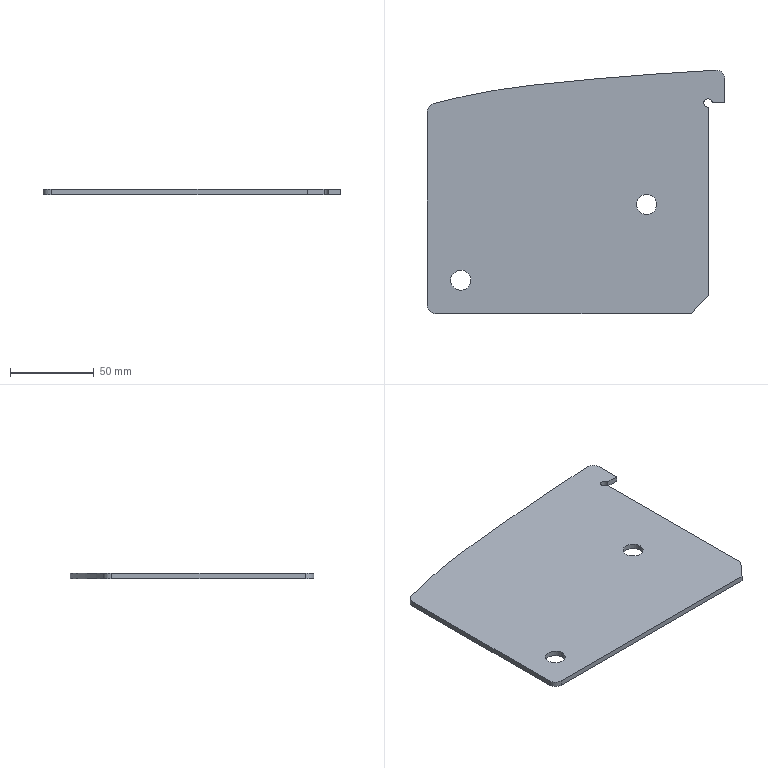Part | SolidWorks | features FlatPattern 1, SMBaseFlange 1, SheetMetal 1 | 1 solid | 19 faces | box 177.818 x 145.585 x 3.2 mm | volume 73602 mm3 | cylinder 11 | plane 8 | commonest cylinder face diameters 12 x4 10 x3 5 x2 796 x1 3976 x1
STEP:
#1=CARTESIAN_POINT('',(-150.,781.7,3.2));
#2=VERTEX_POINT('',#1);
#3=CARTESIAN_POINT('',(-138.,781.7,3.2));
#4=VERTEX_POINT('',#3);
#5=CARTESIAN_POINT('',(-144.,781.7,3.2));
#6=DIRECTION('',(0.,0.,1.));
#7=DIRECTION('',(1.,0.,0.));
#8=AXIS2_PLACEMENT_3D('',#5,#6,#7);
#9=CIRCLE('',#8,6.);
#10=EDGE_CURVE('',#2,#4,#9,.T.);
#11=ORIENTED_EDGE('',*,*,#10,.T.);
#12=CARTESIAN_POINT('',(-138.,781.7,0.));
#13=VERTEX_POINT('',#12);
#14=CARTESIAN_POINT('',(-138.,781.7,3.2));
#15=DIRECTION('',(0.,0.,-1.));
#16=VECTOR('',#15,1000.);
#17=LINE('',#14,#16);
#18=EDGE_CURVE('',#4,#13,#17,.T.);
#19=ORIENTED_EDGE('',*,*,#18,.T.);
#20=CARTESIAN_POINT('',(-150.,781.7,0.));
#21=VERTEX_POINT('',#20);
#22=CARTESIAN_POINT('',(-144.,781.7,0.));
#23=DIRECTION('',(0.,0.,1.));
#24=DIRECTION('',(1.,0.,0.));
#25=AXIS2_PLACEMENT_3D('',#22,#23,#24);
#26=CIRCLE('',#25,6.);
#27=EDGE_CURVE('',#21,#13,#26,.T.);
#28=ORIENTED_EDGE('',*,*,#27,.F.);
#29=CARTESIAN_POINT('',(-150.,781.7,3.2));
#30=DIRECTION('',(0.,0.,-1.));
#31=VECTOR('',#30,1000.);
#32=LINE('',#29,#31);
#33=EDGE_CURVE('',#2,#21,#32,.T.);
#34=ORIENTED_EDGE('',*,*,#33,.F.);
#35=EDGE_LOOP('',(#11,#19,#28,#34));
#36=FACE_OUTER_BOUND('',#35,.T.);
#37=CARTESIAN_POINT('',(-144.,781.7,3.2));
#38=DIRECTION('',(0.,0.,-1.));
#39=DIRECTION('',(-1.,0.,0.));
#40=AXIS2_PLACEMENT_3D('',#37,#38,#39);
#41=CYLINDRICAL_SURFACE('',#40,6.);
#42=ADVANCED_FACE('',(#36),#41,.F.);
#43=CARTESIAN_POINT('',(-38.896,827.041,3.2));
#44=VERTEX_POINT('',#43);
#45=CARTESIAN_POINT('',(-26.896,827.041,3.2));
#46=VERTEX_POINT('',#45);
#47=CARTESIAN_POINT('',(-32.896,827.041,3.2));
#48=DIRECTION('',(0.,0.,1.));
#49=DIRECTION('',(1.,0.,0.));
#50=AXIS2_PLACEMENT_3D('',#47,#48,#49);
#51=CIRCLE('',#50,6.);
#52=EDGE_CURVE('',#44,#46,#51,.T.);
#53=ORIENTED_EDGE('',*,*,#52,.T.);
#54=CARTESIAN_POINT('',(-26.896,827.041,0.));
#55=VERTEX_POINT('',#54);
#56=CARTESIAN_POINT('',(-26.896,827.041,3.2));
#57=DIRECTION('',(0.,0.,-1.));
#58=VECTOR('',#57,1000.);
#59=LINE('',#56,#58);
#60=EDGE_CURVE('',#46,#55,#59,.T.);
#61=ORIENTED_EDGE('',*,*,#60,.T.);
#62=CARTESIAN_POINT('',(-38.896,827.041,0.));
#63=VERTEX_POINT('',#62);
#64=CARTESIAN_POINT('',(-32.896,827.041,0.));
#65=DIRECTION('',(0.,0.,1.));
#66=DIRECTION('',(1.,0.,0.));
#67=AXIS2_PLACEMENT_3D('',#64,#65,#66);
#68=CIRCLE('',#67,6.);
#69=EDGE_CURVE('',#63,#55,#68,.T.);
#70=ORIENTED_EDGE('',*,*,#69,.F.);
#71=CARTESIAN_POINT('',(-38.896,827.041,3.2));
#72=DIRECTION('',(0.,0.,-1.));
#73=VECTOR('',#72,1000.);
#74=LINE('',#71,#73);
#75=EDGE_CURVE('',#44,#63,#74,.T.);
#76=ORIENTED_EDGE('',*,*,#75,.F.);
#77=EDGE_LOOP('',(#53,#61,#70,#76));
#78=FACE_OUTER_BOUND('',#77,.T.);
#79=CARTESIAN_POINT('',(-32.896,827.041,3.2));
#80=DIRECTION('',(0.,0.,-1.));
#81=DIRECTION('',(-1.,0.,0.));
#82=AXIS2_PLACEMENT_3D('',#79,#80,#81);
#83=CYLINDRICAL_SURFACE('',#82,6.);
#84=ADVANCED_FACE('',(#78),#83,.F.);
#85=CARTESIAN_POINT('',(1.318,887.697,3.2));
#86=VERTEX_POINT('',#85);
#87=CARTESIAN_POINT('',(6.318,887.697,3.2));
#88=VERTEX_POINT('',#87);
#89=CARTESIAN_POINT('',(3.818,887.697,3.2));
#90=DIRECTION('',(0.,0.,-1.));
#91=DIRECTION('',(1.,0.,0.));
#92=AXIS2_PLACEMENT_3D('',#89,#90,#91);
#93=CIRCLE('',#92,2.5);
#94=EDGE_CURVE('',#86,#88,#93,.T.);
#95=ORIENTED_EDGE('',*,*,#94,.F.);
#96=CARTESIAN_POINT('',(1.318,887.697,0.));
#97=VERTEX_POINT('',#96);
#98=CARTESIAN_POINT('',(1.318,887.697,3.2));
#99=DIRECTION('',(0.,0.,-1.));
#100=VECTOR('',#99,1000.);
#101=LINE('',#98,#100);
#102=EDGE_CURVE('',#86,#97,#101,.T.);
#103=ORIENTED_EDGE('',*,*,#102,.T.);
#104=CARTESIAN_POINT('',(6.318,887.697,0.));
#105=VERTEX_POINT('',#104);
#106=CARTESIAN_POINT('',(3.818,887.697,0.));
#107=DIRECTION('',(0.,0.,-1.));
#108=DIRECTION('',(1.,0.,0.));
#109=AXIS2_PLACEMENT_3D('',#106,#107,#108);
#110=CIRCLE('',#109,2.5);
#111=EDGE_CURVE('',#97,#105,#110,.T.);
#112=ORIENTED_EDGE('',*,*,#111,.T.);
#113=CARTESIAN_POINT('',(6.318,887.697,3.2));
#114=DIRECTION('',(0.,0.,-1.));
#115=VECTOR('',#114,1000.);
#116=LINE('',#113,#115);
#117=EDGE_CURVE('',#88,#105,#116,.T.);
#118=ORIENTED_EDGE('',*,*,#117,.F.);
#119=EDGE_LOOP('',(#95,#103,#112,#118));
#120=FACE_OUTER_BOUND('',#119,.T.);
#121=CARTESIAN_POINT('',(3.818,887.697,3.2));
#122=DIRECTION('',(0.,0.,-1.));
#123=DIRECTION('',(-1.,0.,0.));
#124=AXIS2_PLACEMENT_3D('',#121,#122,#123);
#125=CYLINDRICAL_SURFACE('',#124,2.5);
#126=ADVANCED_FACE('',(#120),#125,.F.);
#127=ORIENTED_EDGE('',*,*,#52,.F.);
#128=CARTESIAN_POINT('',(-32.896,827.041,3.2));
#129=DIRECTION('',(0.,0.,1.));
#130=DIRECTION('',(1.,0.,0.));
#131=AXIS2_PLACEMENT_3D('',#128,#129,#130);
#132=CIRCLE('',#131,6.);
#133=EDGE_CURVE('',#46,#44,#132,.T.);
#134=ORIENTED_EDGE('',*,*,#133,.F.);
#135=EDGE_LOOP('',(#127,#134));
#136=FACE_BOUND('',#135,.T.);
#137=CARTESIAN_POINT('',(13.818,887.697,3.2));
#138=VERTEX_POINT('',#137);
#139=CARTESIAN_POINT('',(13.818,902.285,3.2));
#140=VERTEX_POINT('',#139);
#141=CARTESIAN_POINT('',(13.818,887.697,3.2));
#142=DIRECTION('',(0.,1.,0.));
#143=VECTOR('',#142,1000.);
#144=LINE('',#141,#143);
#145=EDGE_CURVE('',#138,#140,#144,.T.);
#146=ORIENTED_EDGE('',*,*,#145,.T.);
#147=CARTESIAN_POINT('',(8.551,907.278,3.2));
#148=VERTEX_POINT('',#147);
#149=CARTESIAN_POINT('',(8.818,902.285,3.2));
#150=DIRECTION('',(0.,0.,1.));
#151=DIRECTION('',(1.,0.,0.));
#152=AXIS2_PLACEMENT_3D('',#149,#150,#151);
#153=CIRCLE('',#152,5.);
#154=EDGE_CURVE('',#140,#148,#153,.T.);
#155=ORIENTED_EDGE('',*,*,#154,.T.);
#156=CARTESIAN_POINT('',(-101.22,898.356,3.2));
#157=VERTEX_POINT('',#156);
#158=CARTESIAN_POINT('',(114.664,-1077.888,3.2));
#159=DIRECTION('',(0.,0.,1.));
#160=DIRECTION('',(1.,0.,0.));
#161=AXIS2_PLACEMENT_3D('',#158,#159,#160);
#162=CIRCLE('',#161,1988.);
#163=EDGE_CURVE('',#148,#157,#162,.T.);
#164=ORIENTED_EDGE('',*,*,#163,.T.);
#165=CARTESIAN_POINT('',(-160.285,887.341,3.2));
#166=VERTEX_POINT('',#165);
#167=CARTESIAN_POINT('',(-58.,502.709,3.2));
#168=DIRECTION('',(0.,0.,1.));
#169=DIRECTION('',(1.,0.,0.));
#170=AXIS2_PLACEMENT_3D('',#167,#168,#169);
#171=CIRCLE('',#170,398.);
#172=EDGE_CURVE('',#157,#166,#171,.T.);
#173=ORIENTED_EDGE('',*,*,#172,.T.);
#174=CARTESIAN_POINT('',(-164.,882.509,3.2));
#175=VERTEX_POINT('',#174);
#176=CARTESIAN_POINT('',(-159.,882.509,3.2));
#177=DIRECTION('',(0.,0.,1.));
#178=DIRECTION('',(-1.,0.,0.));
#179=AXIS2_PLACEMENT_3D('',#176,#177,#178);
#180=CIRCLE('',#179,5.);
#181=EDGE_CURVE('',#166,#175,#180,.T.);
#182=ORIENTED_EDGE('',*,*,#181,.T.);
#183=CARTESIAN_POINT('',(-164.,766.7,3.2));
#184=VERTEX_POINT('',#183);
#185=CARTESIAN_POINT('',(-164.,766.7,3.2));
#186=DIRECTION('',(0.,-1.,0.));
#187=VECTOR('',#186,1000.);
#188=LINE('',#185,#187);
#189=EDGE_CURVE('',#175,#184,#188,.T.);
#190=ORIENTED_EDGE('',*,*,#189,.T.);
#191=CARTESIAN_POINT('',(-159.,761.7,3.2));
#192=VERTEX_POINT('',#191);
#193=CARTESIAN_POINT('',(-159.,766.7,3.2));
#194=DIRECTION('',(0.,0.,1.));
#195=DIRECTION('',(-1.,0.,0.));
#196=AXIS2_PLACEMENT_3D('',#193,#194,#195);
#197=CIRCLE('',#196,5.);
#198=EDGE_CURVE('',#184,#192,#197,.T.);
#199=ORIENTED_EDGE('',*,*,#198,.T.);
#200=CARTESIAN_POINT('',(-6.182,761.7,3.2));
#201=VERTEX_POINT('',#200);
#202=CARTESIAN_POINT('',(-6.182,761.7,3.2));
#203=DIRECTION('',(1.,0.,0.));
#204=VECTOR('',#203,1000.);
#205=LINE('',#202,#204);
#206=EDGE_CURVE('',#192,#201,#205,.T.);
#207=ORIENTED_EDGE('',*,*,#206,.T.);
#208=CARTESIAN_POINT('',(3.818,772.697,3.2));
#209=VERTEX_POINT('',#208);
#210=CARTESIAN_POINT('',(3.818,772.697,3.2));
#211=DIRECTION('',(0.6728,0.7398,0.));
#212=VECTOR('',#211,1000.);
#213=LINE('',#210,#212);
#214=EDGE_CURVE('',#201,#209,#213,.T.);
#215=ORIENTED_EDGE('',*,*,#214,.T.);
#216=CARTESIAN_POINT('',(3.818,885.197,3.2));
#217=VERTEX_POINT('',#216);
#218=CARTESIAN_POINT('',(3.818,885.197,3.2));
#219=DIRECTION('',(0.,1.,0.));
#220=VECTOR('',#219,1000.);
#221=LINE('',#218,#220);
#222=EDGE_CURVE('',#209,#217,#221,.T.);
#223=ORIENTED_EDGE('',*,*,#222,.T.);
#224=CARTESIAN_POINT('',(3.818,887.697,3.2));
#225=DIRECTION('',(0.,0.,-1.));
#226=DIRECTION('',(1.,0.,0.));
#227=AXIS2_PLACEMENT_3D('',#224,#225,#226);
#228=CIRCLE('',#227,2.5);
#229=EDGE_CURVE('',#217,#86,#228,.T.);
#230=ORIENTED_EDGE('',*,*,#229,.T.);
#231=ORIENTED_EDGE('',*,*,#94,.T.);
#232=CARTESIAN_POINT('',(6.318,887.697,3.2));
#233=DIRECTION('',(1.,0.,0.));
#234=VECTOR('',#233,1000.);
#235=LINE('',#232,#234);
#236=EDGE_CURVE('',#88,#138,#235,.T.);
#237=ORIENTED_EDGE('',*,*,#236,.T.);
#238=EDGE_LOOP('',(#146,#155,#164,#173,#182,#190,#199,#207,#215,#223,#230,#231,#237));
#239=FACE_OUTER_BOUND('',#238,.T.);
#240=ORIENTED_EDGE('',*,*,#10,.F.);
#241=CARTESIAN_POINT('',(-144.,781.7,3.2));
#242=DIRECTION('',(0.,0.,1.));
#243=DIRECTION('',(1.,0.,0.));
#244=AXIS2_PLACEMENT_3D('',#241,#242,#243);
#245=CIRCLE('',#244,6.);
#246=EDGE_CURVE('',#4,#2,#245,.T.);
#247=ORIENTED_EDGE('',*,*,#246,.F.);
#248=EDGE_LOOP('',(#240,#247));
#249=FACE_BOUND('',#248,.T.);
#250=CARTESIAN_POINT('',(8.818,902.285,3.2));
#251=DIRECTION('',(0.,0.,1.));
#252=DIRECTION('',(1.,0.,0.));
#253=AXIS2_PLACEMENT_3D('',#250,#251,#252);
#254=PLANE('',#253);
#255=ADVANCED_FACE('',(#136,#239,#249),#254,.T.);
#256=CARTESIAN_POINT('',(13.818,887.697,0.));
#257=VERTEX_POINT('',#256);
#258=CARTESIAN_POINT('',(13.818,902.285,0.));
#259=VERTEX_POINT('',#258);
#260=CARTESIAN_POINT('',(13.818,887.697,0.));
#261=DIRECTION('',(0.,1.,0.));
#262=VECTOR('',#261,1000.);
#263=LINE('',#260,#262);
#264=EDGE_CURVE('',#257,#259,#263,.T.);
#265=ORIENTED_EDGE('',*,*,#264,.F.);
#266=CARTESIAN_POINT('',(6.318,887.697,0.));
#267=DIRECTION('',(1.,0.,0.));
#268=VECTOR('',#267,1000.);
#269=LINE('',#266,#268);
#270=EDGE_CURVE('',#105,#257,#269,.T.);
#271=ORIENTED_EDGE('',*,*,#270,.F.);
#272=ORIENTED_EDGE('',*,*,#111,.F.);
#273=CARTESIAN_POINT('',(3.818,885.197,0.));
#274=VERTEX_POINT('',#273);
#275=CARTESIAN_POINT('',(3.818,887.697,0.));
#276=DIRECTION('',(0.,0.,-1.));
#277=DIRECTION('',(1.,0.,0.));
#278=AXIS2_PLACEMENT_3D('',#275,#276,#277);
#279=CIRCLE('',#278,2.5);
#280=EDGE_CURVE('',#274,#97,#279,.T.);
#281=ORIENTED_EDGE('',*,*,#280,.F.);
#282=CARTESIAN_POINT('',(3.818,772.697,0.));
#283=VERTEX_POINT('',#282);
#284=CARTESIAN_POINT('',(3.818,885.197,0.));
#285=DIRECTION('',(0.,1.,0.));
#286=VECTOR('',#285,1000.);
#287=LINE('',#284,#286);
#288=EDGE_CURVE('',#283,#274,#287,.T.);
#289=ORIENTED_EDGE('',*,*,#288,.F.);
#290=CARTESIAN_POINT('',(-6.182,761.7,0.));
#291=VERTEX_POINT('',#290);
#292=CARTESIAN_POINT('',(3.818,772.697,0.));
#293=DIRECTION('',(0.6728,0.7398,0.));
#294=VECTOR('',#293,1000.);
#295=LINE('',#292,#294);
#296=EDGE_CURVE('',#291,#283,#295,.T.);
#297=ORIENTED_EDGE('',*,*,#296,.F.);
#298=CARTESIAN_POINT('',(-159.,761.7,0.));
#299=VERTEX_POINT('',#298);
#300=CARTESIAN_POINT('',(-6.182,761.7,0.));
#301=DIRECTION('',(1.,0.,0.));
#302=VECTOR('',#301,1000.);
#303=LINE('',#300,#302);
#304=EDGE_CURVE('',#299,#291,#303,.T.);
#305=ORIENTED_EDGE('',*,*,#304,.F.);
#306=CARTESIAN_POINT('',(-164.,766.7,0.));
#307=VERTEX_POINT('',#306);
#308=CARTESIAN_POINT('',(-159.,766.7,0.));
#309=DIRECTION('',(0.,0.,1.));
#310=DIRECTION('',(-1.,0.,0.));
#311=AXIS2_PLACEMENT_3D('',#308,#309,#310);
#312=CIRCLE('',#311,5.);
#313=EDGE_CURVE('',#307,#299,#312,.T.);
#314=ORIENTED_EDGE('',*,*,#313,.F.);
#315=CARTESIAN_POINT('',(-164.,882.509,0.));
#316=VERTEX_POINT('',#315);
#317=CARTESIAN_POINT('',(-164.,766.7,0.));
#318=DIRECTION('',(0.,-1.,0.));
#319=VECTOR('',#318,1000.);
#320=LINE('',#317,#319);
#321=EDGE_CURVE('',#316,#307,#320,.T.);
#322=ORIENTED_EDGE('',*,*,#321,.F.);
#323=CARTESIAN_POINT('',(-160.285,887.341,0.));
#324=VERTEX_POINT('',#323);
#325=CARTESIAN_POINT('',(-159.,882.509,0.));
#326=DIRECTION('',(0.,0.,1.));
#327=DIRECTION('',(-1.,0.,0.));
#328=AXIS2_PLACEMENT_3D('',#325,#326,#327);
#329=CIRCLE('',#328,5.);
#330=EDGE_CURVE('',#324,#316,#329,.T.);
#331=ORIENTED_EDGE('',*,*,#330,.F.);
#332=CARTESIAN_POINT('',(-101.22,898.356,0.));
#333=VERTEX_POINT('',#332);
#334=CARTESIAN_POINT('',(-58.,502.709,0.));
#335=DIRECTION('',(0.,0.,1.));
#336=DIRECTION('',(1.,0.,0.));
#337=AXIS2_PLACEMENT_3D('',#334,#335,#336);
#338=CIRCLE('',#337,398.);
#339=EDGE_CURVE('',#333,#324,#338,.T.);
#340=ORIENTED_EDGE('',*,*,#339,.F.);
#341=CARTESIAN_POINT('',(8.551,907.278,0.));
#342=VERTEX_POINT('',#341);
#343=CARTESIAN_POINT('',(114.664,-1077.888,0.));
#344=DIRECTION('',(0.,0.,1.));
#345=DIRECTION('',(1.,0.,0.));
#346=AXIS2_PLACEMENT_3D('',#343,#344,#345);
#347=CIRCLE('',#346,1988.);
#348=EDGE_CURVE('',#342,#333,#347,.T.);
#349=ORIENTED_EDGE('',*,*,#348,.F.);
#350=CARTESIAN_POINT('',(8.818,902.285,0.));
#351=DIRECTION('',(0.,0.,1.));
#352=DIRECTION('',(1.,0.,0.));
#353=AXIS2_PLACEMENT_3D('',#350,#351,#352);
#354=CIRCLE('',#353,5.);
#355=EDGE_CURVE('',#259,#342,#354,.T.);
#356=ORIENTED_EDGE('',*,*,#355,.F.);
#357=EDGE_LOOP('',(#265,#271,#272,#281,#289,#297,#305,#314,#322,#331,#340,#349,#356));
#358=FACE_OUTER_BOUND('',#357,.T.);
#359=ORIENTED_EDGE('',*,*,#69,.T.);
#360=CARTESIAN_POINT('',(-32.896,827.041,0.));
#361=DIRECTION('',(0.,0.,1.));
#362=DIRECTION('',(1.,0.,0.));
#363=AXIS2_PLACEMENT_3D('',#360,#361,#362);
#364=CIRCLE('',#363,6.);
#365=EDGE_CURVE('',#55,#63,#364,.T.);
#366=ORIENTED_EDGE('',*,*,#365,.T.);
#367=EDGE_LOOP('',(#359,#366));
#368=FACE_BOUND('',#367,.T.);
#369=ORIENTED_EDGE('',*,*,#27,.T.);
#370=CARTESIAN_POINT('',(-144.,781.7,0.));
#371=DIRECTION('',(0.,0.,1.));
#372=DIRECTION('',(1.,0.,0.));
#373=AXIS2_PLACEMENT_3D('',#370,#371,#372);
#374=CIRCLE('',#373,6.);
#375=EDGE_CURVE('',#13,#21,#374,.T.);
#376=ORIENTED_EDGE('',*,*,#375,.T.);
#377=EDGE_LOOP('',(#369,#376));
#378=FACE_BOUND('',#377,.T.);
#379=CARTESIAN_POINT('',(8.818,902.285,0.));
#380=DIRECTION('',(0.,0.,1.));
#381=DIRECTION('',(1.,0.,0.));
#382=AXIS2_PLACEMENT_3D('',#379,#380,#381);
#383=PLANE('',#382);
#384=ADVANCED_FACE('',(#358,#368,#378),#383,.F.);
#385=ORIENTED_EDGE('',*,*,#264,.T.);
#386=CARTESIAN_POINT('',(13.818,902.285,3.2));
#387=DIRECTION('',(0.,0.,-1.));
#388=VECTOR('',#387,1000.);
#389=LINE('',#386,#388);
#390=EDGE_CURVE('',#140,#259,#389,.T.);
#391=ORIENTED_EDGE('',*,*,#390,.F.);
#392=ORIENTED_EDGE('',*,*,#145,.F.);
#393=CARTESIAN_POINT('',(13.818,887.697,3.2));
#394=DIRECTION('',(0.,0.,-1.));
#395=VECTOR('',#394,1000.);
#396=LINE('',#393,#395);
#397=EDGE_CURVE('',#138,#257,#396,.T.);
#398=ORIENTED_EDGE('',*,*,#397,.T.);
#399=EDGE_LOOP('',(#385,#391,#392,#398));
#400=FACE_OUTER_BOUND('',#399,.T.);
#401=CARTESIAN_POINT('',(13.818,887.697,3.2));
#402=DIRECTION('',(-1.,0.,0.));
#403=DIRECTION('',(0.,0.,1.));
#404=AXIS2_PLACEMENT_3D('',#401,#402,#403);
#405=PLANE('',#404);
#406=ADVANCED_FACE('',(#400),#405,.F.);
#407=ORIENTED_EDGE('',*,*,#355,.T.);
#408=CARTESIAN_POINT('',(8.551,907.278,3.2));
#409=DIRECTION('',(0.,0.,-1.));
#410=VECTOR('',#409,1000.);
#411=LINE('',#408,#410);
#412=EDGE_CURVE('',#148,#342,#411,.T.);
#413=ORIENTED_EDGE('',*,*,#412,.F.);
#414=ORIENTED_EDGE('',*,*,#154,.F.);
#415=ORIENTED_EDGE('',*,*,#390,.T.);
#416=EDGE_LOOP('',(#407,#413,#414,#415));
#417=FACE_OUTER_BOUND('',#416,.T.);
#418=CARTESIAN_POINT('',(8.818,902.285,3.2));
#419=DIRECTION('',(0.,0.,-1.));
#420=DIRECTION('',(-1.,0.,0.));
#421=AXIS2_PLACEMENT_3D('',#418,#419,#420);
#422=CYLINDRICAL_SURFACE('',#421,5.);
#423=ADVANCED_FACE('',(#417),#422,.T.);
#424=ORIENTED_EDGE('',*,*,#348,.T.);
#425=CARTESIAN_POINT('',(-101.22,898.356,3.2));
#426=DIRECTION('',(0.,0.,-1.));
#427=VECTOR('',#426,1000.);
#428=LINE('',#425,#427);
#429=EDGE_CURVE('',#157,#333,#428,.T.);
#430=ORIENTED_EDGE('',*,*,#429,.F.);
#431=ORIENTED_EDGE('',*,*,#163,.F.);
#432=ORIENTED_EDGE('',*,*,#412,.T.);
#433=EDGE_LOOP('',(#424,#430,#431,#432));
#434=FACE_OUTER_BOUND('',#433,.T.);
#435=CARTESIAN_POINT('',(114.664,-1077.888,3.2));
#436=DIRECTION('',(0.,0.,-1.));
#437=DIRECTION('',(-1.,0.,0.));
#438=AXIS2_PLACEMENT_3D('',#435,#436,#437);
#439=CYLINDRICAL_SURFACE('',#438,1988.);
#440=ADVANCED_FACE('',(#434),#439,.T.);
#441=ORIENTED_EDGE('',*,*,#339,.T.);
#442=CARTESIAN_POINT('',(-160.285,887.341,3.2));
#443=DIRECTION('',(0.,0.,-1.));
#444=VECTOR('',#443,1000.);
#445=LINE('',#442,#444);
#446=EDGE_CURVE('',#166,#324,#445,.T.);
#447=ORIENTED_EDGE('',*,*,#446,.F.);
#448=ORIENTED_EDGE('',*,*,#172,.F.);
#449=ORIENTED_EDGE('',*,*,#429,.T.);
#450=EDGE_LOOP('',(#441,#447,#448,#449));
#451=FACE_OUTER_BOUND('',#450,.T.);
#452=CARTESIAN_POINT('',(-58.,502.709,3.2));
#453=DIRECTION('',(0.,0.,-1.));
#454=DIRECTION('',(-1.,0.,0.));
#455=AXIS2_PLACEMENT_3D('',#452,#453,#454);
#456=CYLINDRICAL_SURFACE('',#455,398.);
#457=ADVANCED_FACE('',(#451),#456,.T.);
#458=ORIENTED_EDGE('',*,*,#330,.T.);
#459=CARTESIAN_POINT('',(-164.,882.509,3.2));
#460=DIRECTION('',(0.,0.,-1.));
#461=VECTOR('',#460,1000.);
#462=LINE('',#459,#461);
#463=EDGE_CURVE('',#175,#316,#462,.T.);
#464=ORIENTED_EDGE('',*,*,#463,.F.);
#465=ORIENTED_EDGE('',*,*,#181,.F.);
#466=ORIENTED_EDGE('',*,*,#446,.T.);
#467=EDGE_LOOP('',(#458,#464,#465,#466));
#468=FACE_OUTER_BOUND('',#467,.T.);
#469=CARTESIAN_POINT('',(-159.,882.509,3.2));
#470=DIRECTION('',(0.,0.,-1.));
#471=DIRECTION('',(-1.,0.,0.));
#472=AXIS2_PLACEMENT_3D('',#469,#470,#471);
#473=CYLINDRICAL_SURFACE('',#472,5.);
#474=ADVANCED_FACE('',(#468),#473,.T.);
#475=ORIENTED_EDGE('',*,*,#321,.T.);
#476=CARTESIAN_POINT('',(-164.,766.7,3.2));
#477=DIRECTION('',(0.,0.,-1.));
#478=VECTOR('',#477,1000.);
#479=LINE('',#476,#478);
#480=EDGE_CURVE('',#184,#307,#479,.T.);
#481=ORIENTED_EDGE('',*,*,#480,.F.);
#482=ORIENTED_EDGE('',*,*,#189,.F.);
#483=ORIENTED_EDGE('',*,*,#463,.T.);
#484=EDGE_LOOP('',(#475,#481,#482,#483));
#485=FACE_OUTER_BOUND('',#484,.T.);
#486=CARTESIAN_POINT('',(-164.,766.7,3.2));
#487=DIRECTION('',(1.,0.,0.));
#488=DIRECTION('',(0.,0.,-1.));
#489=AXIS2_PLACEMENT_3D('',#486,#487,#488);
#490=PLANE('',#489);
#491=ADVANCED_FACE('',(#485),#490,.F.);
#492=ORIENTED_EDGE('',*,*,#313,.T.);
#493=CARTESIAN_POINT('',(-159.,761.7,3.2));
#494=DIRECTION('',(0.,0.,-1.));
#495=VECTOR('',#494,1000.);
#496=LINE('',#493,#495);
#497=EDGE_CURVE('',#192,#299,#496,.T.);
#498=ORIENTED_EDGE('',*,*,#497,.F.);
#499=ORIENTED_EDGE('',*,*,#198,.F.);
#500=ORIENTED_EDGE('',*,*,#480,.T.);
#501=EDGE_LOOP('',(#492,#498,#499,#500));
#502=FACE_OUTER_BOUND('',#501,.T.);
#503=CARTESIAN_POINT('',(-159.,766.7,3.2));
#504=DIRECTION('',(0.,0.,-1.));
#505=DIRECTION('',(-1.,0.,0.));
#506=AXIS2_PLACEMENT_3D('',#503,#504,#505);
#507=CYLINDRICAL_SURFACE('',#506,5.);
#508=ADVANCED_FACE('',(#502),#507,.T.);
#509=ORIENTED_EDGE('',*,*,#304,.T.);
#510=CARTESIAN_POINT('',(-6.182,761.7,3.2));
#511=DIRECTION('',(0.,0.,-1.));
#512=VECTOR('',#511,1000.);
#513=LINE('',#510,#512);
#514=EDGE_CURVE('',#201,#291,#513,.T.);
#515=ORIENTED_EDGE('',*,*,#514,.F.);
#516=ORIENTED_EDGE('',*,*,#206,.F.);
#517=ORIENTED_EDGE('',*,*,#497,.T.);
#518=EDGE_LOOP('',(#509,#515,#516,#517));
#519=FACE_OUTER_BOUND('',#518,.T.);
#520=CARTESIAN_POINT('',(-6.182,761.7,3.2));
#521=DIRECTION('',(0.,1.,0.));
#522=DIRECTION('',(0.,0.,1.));
#523=AXIS2_PLACEMENT_3D('',#520,#521,#522);
#524=PLANE('',#523);
#525=ADVANCED_FACE('',(#519),#524,.F.);
#526=ORIENTED_EDGE('',*,*,#296,.T.);
#527=CARTESIAN_POINT('',(3.818,772.697,3.2));
#528=DIRECTION('',(0.,0.,-1.));
#529=VECTOR('',#528,1000.);
#530=LINE('',#527,#529);
#531=EDGE_CURVE('',#209,#283,#530,.T.);
#532=ORIENTED_EDGE('',*,*,#531,.F.);
#533=ORIENTED_EDGE('',*,*,#214,.F.);
#534=ORIENTED_EDGE('',*,*,#514,.T.);
#535=EDGE_LOOP('',(#526,#532,#533,#534));
#536=FACE_OUTER_BOUND('',#535,.T.);
#537=CARTESIAN_POINT('',(3.818,772.697,3.2));
#538=DIRECTION('',(-0.7398,0.6728,0.));
#539=DIRECTION('',(-0.6728,-0.7398,0.));
#540=AXIS2_PLACEMENT_3D('',#537,#538,#539);
#541=PLANE('',#540);
#542=ADVANCED_FACE('',(#536),#541,.F.);
#543=ORIENTED_EDGE('',*,*,#288,.T.);
#544=CARTESIAN_POINT('',(3.818,885.197,3.2));
#545=DIRECTION('',(0.,0.,-1.));
#546=VECTOR('',#545,1000.);
#547=LINE('',#544,#546);
#548=EDGE_CURVE('',#217,#274,#547,.T.);
#549=ORIENTED_EDGE('',*,*,#548,.F.);
#550=ORIENTED_EDGE('',*,*,#222,.F.);
#551=ORIENTED_EDGE('',*,*,#531,.T.);
#552=EDGE_LOOP('',(#543,#549,#550,#551));
#553=FACE_OUTER_BOUND('',#552,.T.);
#554=CARTESIAN_POINT('',(3.818,885.197,3.2));
#555=DIRECTION('',(-1.,0.,0.));
#556=DIRECTION('',(0.,-1.,0.));
#557=AXIS2_PLACEMENT_3D('',#554,#555,#556);
#558=PLANE('',#557);
#559=ADVANCED_FACE('',(#553),#558,.F.);
#560=ORIENTED_EDGE('',*,*,#102,.F.);
#561=ORIENTED_EDGE('',*,*,#229,.F.);
#562=ORIENTED_EDGE('',*,*,#548,.T.);
#563=ORIENTED_EDGE('',*,*,#280,.T.);
#564=EDGE_LOOP('',(#560,#561,#562,#563));
#565=FACE_OUTER_BOUND('',#564,.T.);
#566=CARTESIAN_POINT('',(3.818,887.697,3.2));
#567=DIRECTION('',(0.,0.,-1.));
#568=DIRECTION('',(-1.,0.,0.));
#569=AXIS2_PLACEMENT_3D('',#566,#567,#568);
#570=CYLINDRICAL_SURFACE('',#569,2.5);
#571=ADVANCED_FACE('',(#565),#570,.F.);
#572=ORIENTED_EDGE('',*,*,#270,.T.);
#573=ORIENTED_EDGE('',*,*,#397,.F.);
#574=ORIENTED_EDGE('',*,*,#236,.F.);
#575=ORIENTED_EDGE('',*,*,#117,.T.);
#576=EDGE_LOOP('',(#572,#573,#574,#575));
#577=FACE_OUTER_BOUND('',#576,.T.);
#578=CARTESIAN_POINT('',(6.318,887.697,3.2));
#579=DIRECTION('',(0.,1.,0.));
#580=DIRECTION('',(0.,0.,1.));
#581=AXIS2_PLACEMENT_3D('',#578,#579,#580);
#582=PLANE('',#581);
#583=ADVANCED_FACE('',(#577),#582,.F.);
#584=ORIENTED_EDGE('',*,*,#60,.F.);
#585=ORIENTED_EDGE('',*,*,#133,.T.);
#586=ORIENTED_EDGE('',*,*,#75,.T.);
#587=ORIENTED_EDGE('',*,*,#365,.F.);
#588=EDGE_LOOP('',(#584,#585,#586,#587));
#589=FACE_OUTER_BOUND('',#588,.T.);
#590=CARTESIAN_POINT('',(-32.896,827.041,3.2));
#591=DIRECTION('',(0.,0.,-1.));
#592=DIRECTION('',(-1.,0.,0.));
#593=AXIS2_PLACEMENT_3D('',#590,#591,#592);
#594=CYLINDRICAL_SURFACE('',#593,6.);
#595=ADVANCED_FACE('',(#589),#594,.F.);
#596=ORIENTED_EDGE('',*,*,#18,.F.);
#597=ORIENTED_EDGE('',*,*,#246,.T.);
#598=ORIENTED_EDGE('',*,*,#33,.T.);
#599=ORIENTED_EDGE('',*,*,#375,.F.);
#600=EDGE_LOOP('',(#596,#597,#598,#599));
#601=FACE_OUTER_BOUND('',#600,.T.);
#602=CARTESIAN_POINT('',(-144.,781.7,3.2));
#603=DIRECTION('',(0.,0.,-1.));
#604=DIRECTION('',(-1.,0.,0.));
#605=AXIS2_PLACEMENT_3D('',#602,#603,#604);
#606=CYLINDRICAL_SURFACE('',#605,6.);
#607=ADVANCED_FACE('',(#601),#606,.F.);
#608=CLOSED_SHELL('',(#42,#84,#126,#255,#384,#406,#423,#440,#457,#474,#491,#508,#525,#542,#559,#571,#583,#595,#607));
#609=MANIFOLD_SOLID_BREP('',#608);
#610=CARTESIAN_POINT('',(0.,0.,0.));
#611=DIRECTION('',(0.,0.,1.));
#612=DIRECTION('',(1.,0.,0.));
#613=AXIS2_PLACEMENT_3D('',#610,#611,#612);
#614=(LENGTH_UNIT()NAMED_UNIT(*)SI_UNIT(.MILLI.,.METRE.));
#615=UNCERTAINTY_MEASURE_WITH_UNIT(LENGTH_MEASURE(0.00001),#614,'','');
#616=(NAMED_UNIT(*)PLANE_ANGLE_UNIT()SI_UNIT($,.RADIAN.));
#617=(NAMED_UNIT(*)SI_UNIT($,.STERADIAN.)SOLID_ANGLE_UNIT());
#618=(GEOMETRIC_REPRESENTATION_CONTEXT(3)GLOBAL_UNCERTAINTY_ASSIGNED_CONTEXT((#615))GLOBAL_UNIT_ASSIGNED_CONTEXT((#614,#616,#617))REPRESENTATION_CONTEXT('',''));
#619=ADVANCED_BREP_SHAPE_REPRESENTATION('',(#609,#613),#618);